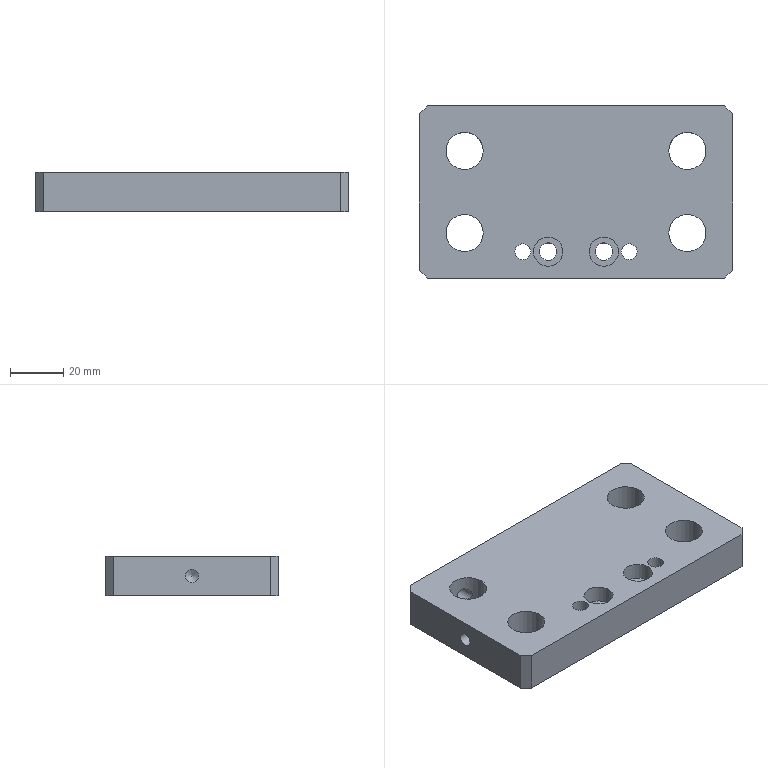Part | NX | features BREP 1 | 1 solid | 26 faces | box 118 x 65 x 15 mm | volume 102149 mm3 | cylinder 13 | plane 12 | cone 1 | commonest cylinder face diameters 14 x4 5 x3 6 x2 6.6 x2 11 x2
STEP:
#1=CARTESIAN_POINT('',(56.,-32.5,0.));
#2=VERTEX_POINT('',#1);
#3=CARTESIAN_POINT('',(59.,-29.5,0.));
#4=VERTEX_POINT('',#3);
#5=CARTESIAN_POINT('',(56.,-32.5,0.));
#6=DIRECTION('',(0.7071,0.7071,0.));
#7=VECTOR('',#6,1000.);
#8=LINE('',#5,#7);
#9=EDGE_CURVE('',#2,#4,#8,.T.);
#10=ORIENTED_EDGE('',*,*,#9,.F.);
#11=CARTESIAN_POINT('',(-56.,-32.5,0.));
#12=VERTEX_POINT('',#11);
#13=CARTESIAN_POINT('',(0.,-32.5,0.));
#14=DIRECTION('',(1.,0.,0.));
#15=VECTOR('',#14,1000.);
#16=LINE('',#13,#15);
#17=EDGE_CURVE('',#12,#2,#16,.T.);
#18=ORIENTED_EDGE('',*,*,#17,.F.);
#19=CARTESIAN_POINT('',(-59.,-29.5,0.));
#20=VERTEX_POINT('',#19);
#21=CARTESIAN_POINT('',(-59.,-29.5,0.));
#22=DIRECTION('',(0.7071,-0.7071,0.));
#23=VECTOR('',#22,1000.);
#24=LINE('',#21,#23);
#25=EDGE_CURVE('',#20,#12,#24,.T.);
#26=ORIENTED_EDGE('',*,*,#25,.F.);
#27=CARTESIAN_POINT('',(-59.,29.5,0.));
#28=VERTEX_POINT('',#27);
#29=CARTESIAN_POINT('',(-59.,0.,0.));
#30=DIRECTION('',(0.,-1.,0.));
#31=VECTOR('',#30,1000.);
#32=LINE('',#29,#31);
#33=EDGE_CURVE('',#28,#20,#32,.T.);
#34=ORIENTED_EDGE('',*,*,#33,.F.);
#35=CARTESIAN_POINT('',(-56.,32.5,0.));
#36=VERTEX_POINT('',#35);
#37=CARTESIAN_POINT('',(-56.,32.5,0.));
#38=DIRECTION('',(-0.7071,-0.7071,0.));
#39=VECTOR('',#38,1000.);
#40=LINE('',#37,#39);
#41=EDGE_CURVE('',#36,#28,#40,.T.);
#42=ORIENTED_EDGE('',*,*,#41,.F.);
#43=CARTESIAN_POINT('',(56.,32.5,0.));
#44=VERTEX_POINT('',#43);
#45=CARTESIAN_POINT('',(0.,32.5,0.));
#46=DIRECTION('',(-1.,0.,0.));
#47=VECTOR('',#46,1000.);
#48=LINE('',#45,#47);
#49=EDGE_CURVE('',#44,#36,#48,.T.);
#50=ORIENTED_EDGE('',*,*,#49,.F.);
#51=CARTESIAN_POINT('',(59.,29.5,0.));
#52=VERTEX_POINT('',#51);
#53=CARTESIAN_POINT('',(59.,29.5,0.));
#54=DIRECTION('',(-0.7071,0.7071,0.));
#55=VECTOR('',#54,1000.);
#56=LINE('',#53,#55);
#57=EDGE_CURVE('',#52,#44,#56,.T.);
#58=ORIENTED_EDGE('',*,*,#57,.F.);
#59=CARTESIAN_POINT('',(59.,0.,0.));
#60=DIRECTION('',(0.,1.,0.));
#61=VECTOR('',#60,1000.);
#62=LINE('',#59,#61);
#63=EDGE_CURVE('',#4,#52,#62,.T.);
#64=ORIENTED_EDGE('',*,*,#63,.F.);
#65=EDGE_LOOP('',(#10,#18,#26,#34,#42,#50,#58,#64));
#66=FACE_BOUND('',#65,.T.);
#67=CARTESIAN_POINT('',(35.,-15.5,0.));
#68=VERTEX_POINT('',#67);
#69=CARTESIAN_POINT('',(42.,-15.5,0.));
#70=DIRECTION('',(0.,0.,-1.));
#71=DIRECTION('',(-1.,0.,0.));
#72=AXIS2_PLACEMENT_3D('',#69,#70,#71);
#73=CIRCLE('',#72,7.);
#74=EDGE_CURVE('',#68,#68,#73,.T.);
#75=ORIENTED_EDGE('',*,*,#74,.F.);
#76=EDGE_LOOP('',(#75));
#77=FACE_BOUND('',#76,.T.);
#78=CARTESIAN_POINT('',(35.,15.5,0.));
#79=VERTEX_POINT('',#78);
#80=CARTESIAN_POINT('',(42.,15.5,0.));
#81=DIRECTION('',(0.,0.,-1.));
#82=DIRECTION('',(-1.,0.,0.));
#83=AXIS2_PLACEMENT_3D('',#80,#81,#82);
#84=CIRCLE('',#83,7.);
#85=EDGE_CURVE('',#79,#79,#84,.T.);
#86=ORIENTED_EDGE('',*,*,#85,.F.);
#87=EDGE_LOOP('',(#86));
#88=FACE_BOUND('',#87,.T.);
#89=CARTESIAN_POINT('',(-49.,15.5,0.));
#90=VERTEX_POINT('',#89);
#91=CARTESIAN_POINT('',(-42.,15.5,0.));
#92=DIRECTION('',(0.,0.,-1.));
#93=DIRECTION('',(-1.,0.,0.));
#94=AXIS2_PLACEMENT_3D('',#91,#92,#93);
#95=CIRCLE('',#94,7.);
#96=EDGE_CURVE('',#90,#90,#95,.T.);
#97=ORIENTED_EDGE('',*,*,#96,.F.);
#98=EDGE_LOOP('',(#97));
#99=FACE_BOUND('',#98,.T.);
#100=CARTESIAN_POINT('',(-49.,-15.5,0.));
#101=VERTEX_POINT('',#100);
#102=CARTESIAN_POINT('',(-42.,-15.5,0.));
#103=DIRECTION('',(0.,0.,-1.));
#104=DIRECTION('',(-1.,0.,0.));
#105=AXIS2_PLACEMENT_3D('',#102,#103,#104);
#106=CIRCLE('',#105,7.);
#107=EDGE_CURVE('',#101,#101,#106,.T.);
#108=ORIENTED_EDGE('',*,*,#107,.F.);
#109=EDGE_LOOP('',(#108));
#110=FACE_BOUND('',#109,.T.);
#111=CARTESIAN_POINT('',(17.,-22.5,0.));
#112=VERTEX_POINT('',#111);
#113=CARTESIAN_POINT('',(20.,-22.5,0.));
#114=DIRECTION('',(0.,0.,-1.));
#115=DIRECTION('',(-1.,0.,0.));
#116=AXIS2_PLACEMENT_3D('',#113,#114,#115);
#117=CIRCLE('',#116,3.);
#118=EDGE_CURVE('',#112,#112,#117,.T.);
#119=ORIENTED_EDGE('',*,*,#118,.F.);
#120=EDGE_LOOP('',(#119));
#121=FACE_BOUND('',#120,.T.);
#122=CARTESIAN_POINT('',(-23.,-22.5,0.));
#123=VERTEX_POINT('',#122);
#124=CARTESIAN_POINT('',(-20.,-22.5,0.));
#125=DIRECTION('',(0.,0.,-1.));
#126=DIRECTION('',(-1.,0.,0.));
#127=AXIS2_PLACEMENT_3D('',#124,#125,#126);
#128=CIRCLE('',#127,3.);
#129=EDGE_CURVE('',#123,#123,#128,.T.);
#130=ORIENTED_EDGE('',*,*,#129,.F.);
#131=EDGE_LOOP('',(#130));
#132=FACE_BOUND('',#131,.T.);
#133=CARTESIAN_POINT('',(13.8,-22.5,0.));
#134=VERTEX_POINT('',#133);
#135=CARTESIAN_POINT('',(10.5,-22.5,0.));
#136=DIRECTION('',(0.,0.,-1.));
#137=DIRECTION('',(1.,0.,0.));
#138=AXIS2_PLACEMENT_3D('',#135,#136,#137);
#139=CIRCLE('',#138,3.3);
#140=EDGE_CURVE('',#134,#134,#139,.T.);
#141=ORIENTED_EDGE('',*,*,#140,.F.);
#142=EDGE_LOOP('',(#141));
#143=FACE_BOUND('',#142,.T.);
#144=CARTESIAN_POINT('',(-7.2,-22.5,0.));
#145=VERTEX_POINT('',#144);
#146=CARTESIAN_POINT('',(-10.5,-22.5,0.));
#147=DIRECTION('',(0.,0.,-1.));
#148=DIRECTION('',(1.,0.,0.));
#149=AXIS2_PLACEMENT_3D('',#146,#147,#148);
#150=CIRCLE('',#149,3.3);
#151=EDGE_CURVE('',#145,#145,#150,.T.);
#152=ORIENTED_EDGE('',*,*,#151,.F.);
#153=EDGE_LOOP('',(#152));
#154=FACE_BOUND('',#153,.T.);
#155=CARTESIAN_POINT('',(0.,0.,0.));
#156=DIRECTION('',(0.,0.,1.));
#157=DIRECTION('',(-1.,0.,0.));
#158=AXIS2_PLACEMENT_3D('',#155,#156,#157);
#159=PLANE('',#158);
#160=ADVANCED_FACE('',(#66,#77,#88,#99,#110,#121,#132,#143,#154),#159,.F.);
#161=CARTESIAN_POINT('',(59.,-29.5,15.));
#162=VERTEX_POINT('',#161);
#163=CARTESIAN_POINT('',(59.,-29.5,15.));
#164=DIRECTION('',(0.,0.,1.));
#165=VECTOR('',#164,1000.);
#166=LINE('',#163,#165);
#167=EDGE_CURVE('',#4,#162,#166,.T.);
#168=ORIENTED_EDGE('',*,*,#167,.F.);
#169=ORIENTED_EDGE('',*,*,#63,.T.);
#170=CARTESIAN_POINT('',(59.,29.5,15.));
#171=VERTEX_POINT('',#170);
#172=CARTESIAN_POINT('',(59.,29.5,15.));
#173=DIRECTION('',(0.,0.,-1.));
#174=VECTOR('',#173,1000.);
#175=LINE('',#172,#174);
#176=EDGE_CURVE('',#171,#52,#175,.T.);
#177=ORIENTED_EDGE('',*,*,#176,.F.);
#178=CARTESIAN_POINT('',(59.,32.5,15.));
#179=DIRECTION('',(0.,1.,0.));
#180=VECTOR('',#179,1000.);
#181=LINE('',#178,#180);
#182=EDGE_CURVE('',#162,#171,#181,.T.);
#183=ORIENTED_EDGE('',*,*,#182,.F.);
#184=EDGE_LOOP('',(#168,#169,#177,#183));
#185=FACE_BOUND('',#184,.T.);
#186=CARTESIAN_POINT('',(59.,32.5,15.));
#187=DIRECTION('',(-1.,0.,0.));
#188=DIRECTION('',(0.,1.,0.));
#189=AXIS2_PLACEMENT_3D('',#186,#187,#188);
#190=PLANE('',#189);
#191=ADVANCED_FACE('',(#185),#190,.F.);
#192=CARTESIAN_POINT('',(56.,-32.5,15.));
#193=VERTEX_POINT('',#192);
#194=CARTESIAN_POINT('',(56.,-32.5,15.));
#195=DIRECTION('',(0.,0.,1.));
#196=VECTOR('',#195,1000.);
#197=LINE('',#194,#196);
#198=EDGE_CURVE('',#2,#193,#197,.T.);
#199=ORIENTED_EDGE('',*,*,#198,.F.);
#200=ORIENTED_EDGE('',*,*,#9,.T.);
#201=ORIENTED_EDGE('',*,*,#167,.T.);
#202=CARTESIAN_POINT('',(59.,-29.5,15.));
#203=DIRECTION('',(0.7071,0.7071,0.));
#204=VECTOR('',#203,1000.);
#205=LINE('',#202,#204);
#206=EDGE_CURVE('',#193,#162,#205,.T.);
#207=ORIENTED_EDGE('',*,*,#206,.F.);
#208=EDGE_LOOP('',(#199,#200,#201,#207));
#209=FACE_BOUND('',#208,.T.);
#210=CARTESIAN_POINT('',(59.,-29.5,15.));
#211=DIRECTION('',(-0.7071,0.7071,0.));
#212=DIRECTION('',(0.7071,0.7071,0.));
#213=AXIS2_PLACEMENT_3D('',#210,#211,#212);
#214=PLANE('',#213);
#215=ADVANCED_FACE('',(#209),#214,.F.);
#216=ORIENTED_EDGE('',*,*,#198,.T.);
#217=CARTESIAN_POINT('',(-56.,-32.5,15.));
#218=VERTEX_POINT('',#217);
#219=CARTESIAN_POINT('',(-59.,-32.5,15.));
#220=DIRECTION('',(1.,0.,0.));
#221=VECTOR('',#220,1000.);
#222=LINE('',#219,#221);
#223=EDGE_CURVE('',#218,#193,#222,.T.);
#224=ORIENTED_EDGE('',*,*,#223,.F.);
#225=CARTESIAN_POINT('',(-56.,-32.5,15.));
#226=DIRECTION('',(0.,0.,1.));
#227=VECTOR('',#226,1000.);
#228=LINE('',#225,#227);
#229=EDGE_CURVE('',#12,#218,#228,.T.);
#230=ORIENTED_EDGE('',*,*,#229,.F.);
#231=ORIENTED_EDGE('',*,*,#17,.T.);
#232=EDGE_LOOP('',(#216,#224,#230,#231));
#233=FACE_BOUND('',#232,.T.);
#234=CARTESIAN_POINT('',(-59.,-32.5,15.));
#235=DIRECTION('',(0.,1.,0.));
#236=DIRECTION('',(0.,0.,-1.));
#237=AXIS2_PLACEMENT_3D('',#234,#235,#236);
#238=PLANE('',#237);
#239=ADVANCED_FACE('',(#233),#238,.F.);
#240=CARTESIAN_POINT('',(-59.,-29.5,15.));
#241=VERTEX_POINT('',#240);
#242=CARTESIAN_POINT('',(-59.,-29.5,15.));
#243=DIRECTION('',(0.,0.,1.));
#244=VECTOR('',#243,1000.);
#245=LINE('',#242,#244);
#246=EDGE_CURVE('',#20,#241,#245,.T.);
#247=ORIENTED_EDGE('',*,*,#246,.F.);
#248=ORIENTED_EDGE('',*,*,#25,.T.);
#249=ORIENTED_EDGE('',*,*,#229,.T.);
#250=CARTESIAN_POINT('',(-56.,-32.5,15.));
#251=DIRECTION('',(0.7071,-0.7071,0.));
#252=VECTOR('',#251,1000.);
#253=LINE('',#250,#252);
#254=EDGE_CURVE('',#241,#218,#253,.T.);
#255=ORIENTED_EDGE('',*,*,#254,.F.);
#256=EDGE_LOOP('',(#247,#248,#249,#255));
#257=FACE_BOUND('',#256,.T.);
#258=CARTESIAN_POINT('',(-56.,-32.5,15.));
#259=DIRECTION('',(0.7071,0.7071,0.));
#260=DIRECTION('',(0.7071,-0.7071,0.));
#261=AXIS2_PLACEMENT_3D('',#258,#259,#260);
#262=PLANE('',#261);
#263=ADVANCED_FACE('',(#257),#262,.F.);
#264=ORIENTED_EDGE('',*,*,#246,.T.);
#265=CARTESIAN_POINT('',(-59.,29.5,15.));
#266=VERTEX_POINT('',#265);
#267=CARTESIAN_POINT('',(-59.,32.5,15.));
#268=DIRECTION('',(0.,-1.,0.));
#269=VECTOR('',#268,1000.);
#270=LINE('',#267,#269);
#271=EDGE_CURVE('',#266,#241,#270,.T.);
#272=ORIENTED_EDGE('',*,*,#271,.F.);
#273=CARTESIAN_POINT('',(-59.,29.5,15.));
#274=DIRECTION('',(0.,0.,1.));
#275=VECTOR('',#274,1000.);
#276=LINE('',#273,#275);
#277=EDGE_CURVE('',#28,#266,#276,.T.);
#278=ORIENTED_EDGE('',*,*,#277,.F.);
#279=ORIENTED_EDGE('',*,*,#33,.T.);
#280=EDGE_LOOP('',(#264,#272,#278,#279));
#281=FACE_BOUND('',#280,.T.);
#282=CARTESIAN_POINT('',(-59.,0.,10.));
#283=VERTEX_POINT('',#282);
#284=CARTESIAN_POINT('',(-59.,0.,7.5));
#285=DIRECTION('',(-1.,0.,0.));
#286=DIRECTION('',(0.,0.,1.));
#287=AXIS2_PLACEMENT_3D('',#284,#285,#286);
#288=CIRCLE('',#287,2.5);
#289=EDGE_CURVE('',#283,#283,#288,.T.);
#290=ORIENTED_EDGE('',*,*,#289,.F.);
#291=EDGE_LOOP('',(#290));
#292=FACE_BOUND('',#291,.T.);
#293=CARTESIAN_POINT('',(-59.,32.5,15.));
#294=DIRECTION('',(1.,0.,0.));
#295=DIRECTION('',(0.,-1.,0.));
#296=AXIS2_PLACEMENT_3D('',#293,#294,#295);
#297=PLANE('',#296);
#298=ADVANCED_FACE('',(#281,#292),#297,.F.);
#299=CARTESIAN_POINT('',(-56.,32.5,15.));
#300=VERTEX_POINT('',#299);
#301=CARTESIAN_POINT('',(-56.,32.5,15.));
#302=DIRECTION('',(0.,0.,1.));
#303=VECTOR('',#302,1000.);
#304=LINE('',#301,#303);
#305=EDGE_CURVE('',#36,#300,#304,.T.);
#306=ORIENTED_EDGE('',*,*,#305,.F.);
#307=ORIENTED_EDGE('',*,*,#41,.T.);
#308=ORIENTED_EDGE('',*,*,#277,.T.);
#309=CARTESIAN_POINT('',(-59.,29.5,15.));
#310=DIRECTION('',(-0.7071,-0.7071,0.));
#311=VECTOR('',#310,1000.);
#312=LINE('',#309,#311);
#313=EDGE_CURVE('',#300,#266,#312,.T.);
#314=ORIENTED_EDGE('',*,*,#313,.F.);
#315=EDGE_LOOP('',(#306,#307,#308,#314));
#316=FACE_BOUND('',#315,.T.);
#317=CARTESIAN_POINT('',(-59.,29.5,15.));
#318=DIRECTION('',(0.7071,-0.7071,0.));
#319=DIRECTION('',(-0.7071,-0.7071,0.));
#320=AXIS2_PLACEMENT_3D('',#317,#318,#319);
#321=PLANE('',#320);
#322=ADVANCED_FACE('',(#316),#321,.F.);
#323=CARTESIAN_POINT('',(56.,32.5,15.));
#324=VERTEX_POINT('',#323);
#325=CARTESIAN_POINT('',(56.,32.5,15.));
#326=DIRECTION('',(0.,0.,1.));
#327=VECTOR('',#326,1000.);
#328=LINE('',#325,#327);
#329=EDGE_CURVE('',#44,#324,#328,.T.);
#330=ORIENTED_EDGE('',*,*,#329,.F.);
#331=ORIENTED_EDGE('',*,*,#49,.T.);
#332=ORIENTED_EDGE('',*,*,#305,.T.);
#333=CARTESIAN_POINT('',(-59.,32.5,15.));
#334=DIRECTION('',(-1.,0.,0.));
#335=VECTOR('',#334,1000.);
#336=LINE('',#333,#335);
#337=EDGE_CURVE('',#324,#300,#336,.T.);
#338=ORIENTED_EDGE('',*,*,#337,.F.);
#339=EDGE_LOOP('',(#330,#331,#332,#338));
#340=FACE_BOUND('',#339,.T.);
#341=CARTESIAN_POINT('',(-38.5,32.5,10.));
#342=VERTEX_POINT('',#341);
#343=CARTESIAN_POINT('',(-38.5,32.5,7.5));
#344=DIRECTION('',(0.,1.,0.));
#345=DIRECTION('',(0.,0.,1.));
#346=AXIS2_PLACEMENT_3D('',#343,#344,#345);
#347=CIRCLE('',#346,2.5);
#348=EDGE_CURVE('',#342,#342,#347,.T.);
#349=ORIENTED_EDGE('',*,*,#348,.F.);
#350=EDGE_LOOP('',(#349));
#351=FACE_BOUND('',#350,.T.);
#352=CARTESIAN_POINT('',(38.5,32.5,10.));
#353=VERTEX_POINT('',#352);
#354=CARTESIAN_POINT('',(38.5,32.5,7.5));
#355=DIRECTION('',(0.,1.,0.));
#356=DIRECTION('',(0.,0.,1.));
#357=AXIS2_PLACEMENT_3D('',#354,#355,#356);
#358=CIRCLE('',#357,2.5);
#359=EDGE_CURVE('',#353,#353,#358,.T.);
#360=ORIENTED_EDGE('',*,*,#359,.F.);
#361=EDGE_LOOP('',(#360));
#362=FACE_BOUND('',#361,.T.);
#363=CARTESIAN_POINT('',(-59.,32.5,15.));
#364=DIRECTION('',(0.,-1.,0.));
#365=DIRECTION('',(0.,0.,1.));
#366=AXIS2_PLACEMENT_3D('',#363,#364,#365);
#367=PLANE('',#366);
#368=ADVANCED_FACE('',(#340,#351,#362),#367,.F.);
#369=ORIENTED_EDGE('',*,*,#176,.T.);
#370=ORIENTED_EDGE('',*,*,#57,.T.);
#371=ORIENTED_EDGE('',*,*,#329,.T.);
#372=CARTESIAN_POINT('',(56.,32.5,15.));
#373=DIRECTION('',(-0.7071,0.7071,0.));
#374=VECTOR('',#373,1000.);
#375=LINE('',#372,#374);
#376=EDGE_CURVE('',#171,#324,#375,.T.);
#377=ORIENTED_EDGE('',*,*,#376,.F.);
#378=EDGE_LOOP('',(#369,#370,#371,#377));
#379=FACE_BOUND('',#378,.T.);
#380=CARTESIAN_POINT('',(56.,32.5,15.));
#381=DIRECTION('',(-0.7071,-0.7071,0.));
#382=DIRECTION('',(-0.7071,0.7071,0.));
#383=AXIS2_PLACEMENT_3D('',#380,#381,#382);
#384=PLANE('',#383);
#385=ADVANCED_FACE('',(#379),#384,.F.);
#386=CARTESIAN_POINT('',(35.,-15.5,15.));
#387=VERTEX_POINT('',#386);
#388=CARTESIAN_POINT('',(42.,-15.5,15.));
#389=DIRECTION('',(0.,0.,-1.));
#390=DIRECTION('',(-1.,0.,0.));
#391=AXIS2_PLACEMENT_3D('',#388,#389,#390);
#392=CIRCLE('',#391,7.);
#393=EDGE_CURVE('',#387,#387,#392,.T.);
#394=ORIENTED_EDGE('',*,*,#393,.F.);
#395=EDGE_LOOP('',(#394));
#396=FACE_BOUND('',#395,.T.);
#397=ORIENTED_EDGE('',*,*,#74,.T.);
#398=EDGE_LOOP('',(#397));
#399=FACE_BOUND('',#398,.T.);
#400=CARTESIAN_POINT('',(42.,-15.5,0.));
#401=DIRECTION('',(0.,0.,-1.));
#402=DIRECTION('',(1.,0.,0.));
#403=AXIS2_PLACEMENT_3D('',#400,#401,#402);
#404=CYLINDRICAL_SURFACE('',#403,7.);
#405=ADVANCED_FACE('',(#396,#399),#404,.F.);
#406=CARTESIAN_POINT('',(35.,15.5,15.));
#407=VERTEX_POINT('',#406);
#408=CARTESIAN_POINT('',(42.,15.5,15.));
#409=DIRECTION('',(0.,0.,-1.));
#410=DIRECTION('',(-1.,0.,0.));
#411=AXIS2_PLACEMENT_3D('',#408,#409,#410);
#412=CIRCLE('',#411,7.);
#413=EDGE_CURVE('',#407,#407,#412,.T.);
#414=ORIENTED_EDGE('',*,*,#413,.F.);
#415=EDGE_LOOP('',(#414));
#416=FACE_BOUND('',#415,.T.);
#417=CARTESIAN_POINT('',(38.5,21.562,5.));
#418=VERTEX_POINT('',#417);
#419=CARTESIAN_POINT('',(37.584,20.964,5.121));
#420=CARTESIAN_POINT('',(38.781,21.8,4.873));
#421=CARTESIAN_POINT('',(40.552,22.412,5.543));
#422=CARTESIAN_POINT('',(41.332,22.458,7.855));
#423=CARTESIAN_POINT('',(40.004,22.31,9.885));
#424=CARTESIAN_POINT('',(38.218,21.475,10.112));
#425=CARTESIAN_POINT('',(37.144,20.573,9.656));
#426=CARTESIAN_POINT('',(36.511,19.877,9.089));
#427=CARTESIAN_POINT('',(36.057,19.211,8.307));
#428=CARTESIAN_POINT('',(35.941,19.007,7.152));
#429=CARTESIAN_POINT('',(36.298,19.588,6.209));
#430=CARTESIAN_POINT('',(36.849,20.272,5.562));
#431=CARTESIAN_POINT('',(37.584,20.964,5.121));
#432=CARTESIAN_POINT('',(38.781,21.8,4.873));
#433=CARTESIAN_POINT('',(40.552,22.412,5.543));
#434=B_SPLINE_CURVE_WITH_KNOTS('',3,(#419,#420,#421,#422,#423,#424,#425,#426,#427,#428,#429,#430,#431,#432,#433),.UNSPECIFIED.,.T.,.F.,(1,1,1,1,1,1,1,1,1,1,1,1,1,1,1,1,1,1,1),(-0.003271,-0.002181,-0.00109,0.,0.002181,0.004362,0.006543,0.008723,0.009814,0.0109,0.01199,0.01309,0.01418,0.01527,0.01636,0.01745,0.01963,0.02181,0.02399),.UNSPECIFIED.);
#435=EDGE_CURVE('',#418,#418,#434,.T.);
#436=ORIENTED_EDGE('',*,*,#435,.F.);
#437=EDGE_LOOP('',(#436));
#438=FACE_BOUND('',#437,.T.);
#439=ORIENTED_EDGE('',*,*,#85,.T.);
#440=EDGE_LOOP('',(#439));
#441=FACE_BOUND('',#440,.T.);
#442=CARTESIAN_POINT('',(42.,15.5,0.));
#443=DIRECTION('',(0.,0.,-1.));
#444=DIRECTION('',(1.,0.,0.));
#445=AXIS2_PLACEMENT_3D('',#442,#443,#444);
#446=CYLINDRICAL_SURFACE('',#445,7.);
#447=ADVANCED_FACE('',(#416,#438,#441),#446,.F.);
#448=CARTESIAN_POINT('',(-49.,15.5,15.));
#449=VERTEX_POINT('',#448);
#450=CARTESIAN_POINT('',(-42.,15.5,15.));
#451=DIRECTION('',(0.,0.,-1.));
#452=DIRECTION('',(-1.,0.,0.));
#453=AXIS2_PLACEMENT_3D('',#450,#451,#452);
#454=CIRCLE('',#453,7.);
#455=EDGE_CURVE('',#449,#449,#454,.T.);
#456=ORIENTED_EDGE('',*,*,#455,.F.);
#457=EDGE_LOOP('',(#456));
#458=FACE_BOUND('',#457,.T.);
#459=CARTESIAN_POINT('',(-38.5,21.562,5.));
#460=VERTEX_POINT('',#459);
#461=CARTESIAN_POINT('',(-40.562,22.415,5.55));
#462=CARTESIAN_POINT('',(-38.777,21.797,4.873));
#463=CARTESIAN_POINT('',(-37.589,20.968,5.119));
#464=CARTESIAN_POINT('',(-36.848,20.271,5.562));
#465=CARTESIAN_POINT('',(-36.297,19.587,6.21));
#466=CARTESIAN_POINT('',(-35.94,19.006,7.157));
#467=CARTESIAN_POINT('',(-36.059,19.213,8.31));
#468=CARTESIAN_POINT('',(-36.514,19.88,9.092));
#469=CARTESIAN_POINT('',(-37.144,20.572,9.655));
#470=CARTESIAN_POINT('',(-38.21,21.469,10.11));
#471=CARTESIAN_POINT('',(-39.988,22.306,9.896));
#472=CARTESIAN_POINT('',(-41.332,22.458,7.866));
#473=CARTESIAN_POINT('',(-40.562,22.415,5.55));
#474=CARTESIAN_POINT('',(-38.777,21.797,4.873));
#475=CARTESIAN_POINT('',(-37.589,20.968,5.119));
#476=B_SPLINE_CURVE_WITH_KNOTS('',3,(#461,#462,#463,#464,#465,#466,#467,#468,#469,#470,#471,#472,#473,#474,#475),.UNSPECIFIED.,.T.,.F.,(1,1,1,1,1,1,1,1,1,1,1,1,1,1,1,1,1,1,1),(-0.006513,-0.004342,-0.002171,0.,0.001085,0.002171,0.003256,0.004342,0.005427,0.006513,0.007598,0.008683,0.01085,0.01303,0.0152,0.01737,0.01845,0.01954,0.02062),.UNSPECIFIED.);
#477=EDGE_CURVE('',#460,#460,#476,.T.);
#478=ORIENTED_EDGE('',*,*,#477,.F.);
#479=EDGE_LOOP('',(#478));
#480=FACE_BOUND('',#479,.T.);
#481=ORIENTED_EDGE('',*,*,#96,.T.);
#482=EDGE_LOOP('',(#481));
#483=FACE_BOUND('',#482,.T.);
#484=CARTESIAN_POINT('',(-42.,15.5,0.));
#485=DIRECTION('',(0.,0.,-1.));
#486=DIRECTION('',(1.,0.,0.));
#487=AXIS2_PLACEMENT_3D('',#484,#485,#486);
#488=CYLINDRICAL_SURFACE('',#487,7.);
#489=ADVANCED_FACE('',(#458,#480,#483),#488,.F.);
#490=CARTESIAN_POINT('',(-49.,-15.5,15.));
#491=VERTEX_POINT('',#490);
#492=CARTESIAN_POINT('',(-42.,-15.5,15.));
#493=DIRECTION('',(0.,0.,-1.));
#494=DIRECTION('',(-1.,0.,0.));
#495=AXIS2_PLACEMENT_3D('',#492,#493,#494);
#496=CIRCLE('',#495,7.);
#497=EDGE_CURVE('',#491,#491,#496,.T.);
#498=ORIENTED_EDGE('',*,*,#497,.F.);
#499=EDGE_LOOP('',(#498));
#500=FACE_BOUND('',#499,.T.);
#501=ORIENTED_EDGE('',*,*,#107,.T.);
#502=EDGE_LOOP('',(#501));
#503=FACE_BOUND('',#502,.T.);
#504=CARTESIAN_POINT('',(-42.,-15.5,0.));
#505=DIRECTION('',(0.,0.,-1.));
#506=DIRECTION('',(1.,0.,0.));
#507=AXIS2_PLACEMENT_3D('',#504,#505,#506);
#508=CYLINDRICAL_SURFACE('',#507,7.);
#509=ADVANCED_FACE('',(#500,#503),#508,.F.);
#510=CARTESIAN_POINT('',(17.,-22.5,15.));
#511=VERTEX_POINT('',#510);
#512=CARTESIAN_POINT('',(20.,-22.5,15.));
#513=DIRECTION('',(0.,0.,-1.));
#514=DIRECTION('',(-1.,0.,0.));
#515=AXIS2_PLACEMENT_3D('',#512,#513,#514);
#516=CIRCLE('',#515,3.);
#517=EDGE_CURVE('',#511,#511,#516,.T.);
#518=ORIENTED_EDGE('',*,*,#517,.F.);
#519=EDGE_LOOP('',(#518));
#520=FACE_BOUND('',#519,.T.);
#521=ORIENTED_EDGE('',*,*,#118,.T.);
#522=EDGE_LOOP('',(#521));
#523=FACE_BOUND('',#522,.T.);
#524=CARTESIAN_POINT('',(20.,-22.5,0.));
#525=DIRECTION('',(0.,0.,-1.));
#526=DIRECTION('',(1.,0.,0.));
#527=AXIS2_PLACEMENT_3D('',#524,#525,#526);
#528=CYLINDRICAL_SURFACE('',#527,3.);
#529=ADVANCED_FACE('',(#520,#523),#528,.F.);
#530=CARTESIAN_POINT('',(-23.,-22.5,15.));
#531=VERTEX_POINT('',#530);
#532=CARTESIAN_POINT('',(-20.,-22.5,15.));
#533=DIRECTION('',(0.,0.,-1.));
#534=DIRECTION('',(-1.,0.,0.));
#535=AXIS2_PLACEMENT_3D('',#532,#533,#534);
#536=CIRCLE('',#535,3.);
#537=EDGE_CURVE('',#531,#531,#536,.T.);
#538=ORIENTED_EDGE('',*,*,#537,.F.);
#539=EDGE_LOOP('',(#538));
#540=FACE_BOUND('',#539,.T.);
#541=ORIENTED_EDGE('',*,*,#129,.T.);
#542=EDGE_LOOP('',(#541));
#543=FACE_BOUND('',#542,.T.);
#544=CARTESIAN_POINT('',(-20.,-22.5,0.));
#545=DIRECTION('',(0.,0.,-1.));
#546=DIRECTION('',(1.,0.,0.));
#547=AXIS2_PLACEMENT_3D('',#544,#545,#546);
#548=CYLINDRICAL_SURFACE('',#547,3.);
#549=ADVANCED_FACE('',(#540,#543),#548,.F.);
#550=ORIENTED_EDGE('',*,*,#140,.T.);
#551=EDGE_LOOP('',(#550));
#552=FACE_BOUND('',#551,.T.);
#553=CARTESIAN_POINT('',(13.8,-22.5,8.6));
#554=VERTEX_POINT('',#553);
#555=CARTESIAN_POINT('',(10.5,-22.5,8.6));
#556=DIRECTION('',(0.,0.,-1.));
#557=DIRECTION('',(1.,0.,0.));
#558=AXIS2_PLACEMENT_3D('',#555,#556,#557);
#559=CIRCLE('',#558,3.3);
#560=EDGE_CURVE('',#554,#554,#559,.T.);
#561=ORIENTED_EDGE('',*,*,#560,.F.);
#562=EDGE_LOOP('',(#561));
#563=FACE_BOUND('',#562,.T.);
#564=CARTESIAN_POINT('',(10.5,-22.5,15.));
#565=DIRECTION('',(0.,0.,1.));
#566=DIRECTION('',(-1.,0.,0.));
#567=AXIS2_PLACEMENT_3D('',#564,#565,#566);
#568=CYLINDRICAL_SURFACE('',#567,3.3);
#569=ADVANCED_FACE('',(#552,#563),#568,.F.);
#570=ORIENTED_EDGE('',*,*,#151,.T.);
#571=EDGE_LOOP('',(#570));
#572=FACE_BOUND('',#571,.T.);
#573=CARTESIAN_POINT('',(-7.2,-22.5,8.6));
#574=VERTEX_POINT('',#573);
#575=CARTESIAN_POINT('',(-10.5,-22.5,8.6));
#576=DIRECTION('',(0.,0.,-1.));
#577=DIRECTION('',(1.,0.,0.));
#578=AXIS2_PLACEMENT_3D('',#575,#576,#577);
#579=CIRCLE('',#578,3.3);
#580=EDGE_CURVE('',#574,#574,#579,.T.);
#581=ORIENTED_EDGE('',*,*,#580,.F.);
#582=EDGE_LOOP('',(#581));
#583=FACE_BOUND('',#582,.T.);
#584=CARTESIAN_POINT('',(-10.5,-22.5,15.));
#585=DIRECTION('',(0.,0.,1.));
#586=DIRECTION('',(-1.,0.,0.));
#587=AXIS2_PLACEMENT_3D('',#584,#585,#586);
#588=CYLINDRICAL_SURFACE('',#587,3.3);
#589=ADVANCED_FACE('',(#572,#583),#588,.F.);
#590=ORIENTED_EDGE('',*,*,#271,.T.);
#591=ORIENTED_EDGE('',*,*,#254,.T.);
#592=ORIENTED_EDGE('',*,*,#223,.T.);
#593=ORIENTED_EDGE('',*,*,#206,.T.);
#594=ORIENTED_EDGE('',*,*,#182,.T.);
#595=ORIENTED_EDGE('',*,*,#376,.T.);
#596=ORIENTED_EDGE('',*,*,#337,.T.);
#597=ORIENTED_EDGE('',*,*,#313,.T.);
#598=EDGE_LOOP('',(#590,#591,#592,#593,#594,#595,#596,#597));
#599=FACE_BOUND('',#598,.T.);
#600=ORIENTED_EDGE('',*,*,#393,.T.);
#601=EDGE_LOOP('',(#600));
#602=FACE_BOUND('',#601,.T.);
#603=ORIENTED_EDGE('',*,*,#413,.T.);
#604=EDGE_LOOP('',(#603));
#605=FACE_BOUND('',#604,.T.);
#606=ORIENTED_EDGE('',*,*,#455,.T.);
#607=EDGE_LOOP('',(#606));
#608=FACE_BOUND('',#607,.T.);
#609=ORIENTED_EDGE('',*,*,#497,.T.);
#610=EDGE_LOOP('',(#609));
#611=FACE_BOUND('',#610,.T.);
#612=ORIENTED_EDGE('',*,*,#517,.T.);
#613=EDGE_LOOP('',(#612));
#614=FACE_BOUND('',#613,.T.);
#615=ORIENTED_EDGE('',*,*,#537,.T.);
#616=EDGE_LOOP('',(#615));
#617=FACE_BOUND('',#616,.T.);
#618=CARTESIAN_POINT('',(16.,-22.5,15.));
#619=VERTEX_POINT('',#618);
#620=CARTESIAN_POINT('',(10.5,-22.5,15.));
#621=DIRECTION('',(0.,0.,-1.));
#622=DIRECTION('',(1.,0.,0.));
#623=AXIS2_PLACEMENT_3D('',#620,#621,#622);
#624=CIRCLE('',#623,5.5);
#625=EDGE_CURVE('',#619,#619,#624,.T.);
#626=ORIENTED_EDGE('',*,*,#625,.T.);
#627=EDGE_LOOP('',(#626));
#628=FACE_BOUND('',#627,.T.);
#629=CARTESIAN_POINT('',(-5.,-22.5,15.));
#630=VERTEX_POINT('',#629);
#631=CARTESIAN_POINT('',(-10.5,-22.5,15.));
#632=DIRECTION('',(0.,0.,-1.));
#633=DIRECTION('',(1.,0.,0.));
#634=AXIS2_PLACEMENT_3D('',#631,#632,#633);
#635=CIRCLE('',#634,5.5);
#636=EDGE_CURVE('',#630,#630,#635,.T.);
#637=ORIENTED_EDGE('',*,*,#636,.T.);
#638=EDGE_LOOP('',(#637));
#639=FACE_BOUND('',#638,.T.);
#640=CARTESIAN_POINT('',(0.,0.,15.));
#641=DIRECTION('',(0.,0.,1.));
#642=DIRECTION('',(-1.,0.,0.));
#643=AXIS2_PLACEMENT_3D('',#640,#641,#642);
#644=PLANE('',#643);
#645=ADVANCED_FACE('',(#599,#602,#605,#608,#611,#614,#617,#628,#639),#644,.T.);
#646=CARTESIAN_POINT('',(-44.,0.,10.));
#647=VERTEX_POINT('',#646);
#648=CARTESIAN_POINT('',(-44.,0.,7.5));
#649=DIRECTION('',(-1.,0.,0.));
#650=DIRECTION('',(0.,0.,1.));
#651=AXIS2_PLACEMENT_3D('',#648,#649,#650);
#652=CIRCLE('',#651,2.5);
#653=EDGE_CURVE('',#647,#647,#652,.T.);
#654=ORIENTED_EDGE('',*,*,#653,.F.);
#655=EDGE_LOOP('',(#654));
#656=FACE_BOUND('',#655,.T.);
#657=ORIENTED_EDGE('',*,*,#289,.T.);
#658=EDGE_LOOP('',(#657));
#659=FACE_BOUND('',#658,.T.);
#660=CARTESIAN_POINT('',(-59.,0.,7.5));
#661=DIRECTION('',(-1.,0.,0.));
#662=DIRECTION('',(0.,0.,-1.));
#663=AXIS2_PLACEMENT_3D('',#660,#661,#662);
#664=CYLINDRICAL_SURFACE('',#663,2.5);
#665=ADVANCED_FACE('',(#656,#659),#664,.F.);
#666=ORIENTED_EDGE('',*,*,#477,.T.);
#667=EDGE_LOOP('',(#666));
#668=FACE_BOUND('',#667,.T.);
#669=ORIENTED_EDGE('',*,*,#348,.T.);
#670=EDGE_LOOP('',(#669));
#671=FACE_BOUND('',#670,.T.);
#672=CARTESIAN_POINT('',(-38.5,32.5,7.5));
#673=DIRECTION('',(0.,1.,0.));
#674=DIRECTION('',(0.,0.,-1.));
#675=AXIS2_PLACEMENT_3D('',#672,#673,#674);
#676=CYLINDRICAL_SURFACE('',#675,2.5);
#677=ADVANCED_FACE('',(#668,#671),#676,.F.);
#678=ORIENTED_EDGE('',*,*,#435,.T.);
#679=EDGE_LOOP('',(#678));
#680=FACE_BOUND('',#679,.T.);
#681=ORIENTED_EDGE('',*,*,#359,.T.);
#682=EDGE_LOOP('',(#681));
#683=FACE_BOUND('',#682,.T.);
#684=CARTESIAN_POINT('',(38.5,32.5,7.5));
#685=DIRECTION('',(0.,1.,0.));
#686=DIRECTION('',(0.,0.,-1.));
#687=AXIS2_PLACEMENT_3D('',#684,#685,#686);
#688=CYLINDRICAL_SURFACE('',#687,2.5);
#689=ADVANCED_FACE('',(#680,#683),#688,.F.);
#690=CARTESIAN_POINT('',(16.,-22.5,8.6));
#691=VERTEX_POINT('',#690);
#692=CARTESIAN_POINT('',(10.5,-22.5,8.6));
#693=DIRECTION('',(0.,0.,-1.));
#694=DIRECTION('',(1.,0.,0.));
#695=AXIS2_PLACEMENT_3D('',#692,#693,#694);
#696=CIRCLE('',#695,5.5);
#697=EDGE_CURVE('',#691,#691,#696,.T.);
#698=ORIENTED_EDGE('',*,*,#697,.F.);
#699=EDGE_LOOP('',(#698));
#700=FACE_BOUND('',#699,.T.);
#701=ORIENTED_EDGE('',*,*,#560,.T.);
#702=EDGE_LOOP('',(#701));
#703=FACE_BOUND('',#702,.T.);
#704=CARTESIAN_POINT('',(13.8,-22.5,8.6));
#705=DIRECTION('',(0.,0.,-1.));
#706=DIRECTION('',(1.,0.,0.));
#707=AXIS2_PLACEMENT_3D('',#704,#705,#706);
#708=PLANE('',#707);
#709=ADVANCED_FACE('',(#700,#703),#708,.F.);
#710=CARTESIAN_POINT('',(-5.,-22.5,8.6));
#711=VERTEX_POINT('',#710);
#712=CARTESIAN_POINT('',(-10.5,-22.5,8.6));
#713=DIRECTION('',(0.,0.,-1.));
#714=DIRECTION('',(1.,0.,0.));
#715=AXIS2_PLACEMENT_3D('',#712,#713,#714);
#716=CIRCLE('',#715,5.5);
#717=EDGE_CURVE('',#711,#711,#716,.T.);
#718=ORIENTED_EDGE('',*,*,#717,.F.);
#719=EDGE_LOOP('',(#718));
#720=FACE_BOUND('',#719,.T.);
#721=ORIENTED_EDGE('',*,*,#580,.T.);
#722=EDGE_LOOP('',(#721));
#723=FACE_BOUND('',#722,.T.);
#724=CARTESIAN_POINT('',(-7.2,-22.5,8.6));
#725=DIRECTION('',(0.,0.,-1.));
#726=DIRECTION('',(1.,0.,0.));
#727=AXIS2_PLACEMENT_3D('',#724,#725,#726);
#728=PLANE('',#727);
#729=ADVANCED_FACE('',(#720,#723),#728,.F.);
#730=ORIENTED_EDGE('',*,*,#625,.F.);
#731=EDGE_LOOP('',(#730));
#732=FACE_BOUND('',#731,.T.);
#733=ORIENTED_EDGE('',*,*,#697,.T.);
#734=EDGE_LOOP('',(#733));
#735=FACE_BOUND('',#734,.T.);
#736=CARTESIAN_POINT('',(10.5,-22.5,15.));
#737=DIRECTION('',(0.,0.,1.));
#738=DIRECTION('',(-1.,0.,0.));
#739=AXIS2_PLACEMENT_3D('',#736,#737,#738);
#740=CYLINDRICAL_SURFACE('',#739,5.5);
#741=ADVANCED_FACE('',(#732,#735),#740,.F.);
#742=ORIENTED_EDGE('',*,*,#636,.F.);
#743=EDGE_LOOP('',(#742));
#744=FACE_BOUND('',#743,.T.);
#745=ORIENTED_EDGE('',*,*,#717,.T.);
#746=EDGE_LOOP('',(#745));
#747=FACE_BOUND('',#746,.T.);
#748=CARTESIAN_POINT('',(-10.5,-22.5,15.));
#749=DIRECTION('',(0.,0.,1.));
#750=DIRECTION('',(-1.,0.,0.));
#751=AXIS2_PLACEMENT_3D('',#748,#749,#750);
#752=CYLINDRICAL_SURFACE('',#751,5.5);
#753=ADVANCED_FACE('',(#744,#747),#752,.F.);
#754=CARTESIAN_POINT('',(-42.498,0.,7.5));
#755=VERTEX_POINT('',#754);
#756=VERTEX_LOOP('',#755);
#757=FACE_BOUND('',#756,.T.);
#758=ORIENTED_EDGE('',*,*,#653,.T.);
#759=EDGE_LOOP('',(#758));
#760=FACE_BOUND('',#759,.T.);
#761=CARTESIAN_POINT('',(-44.,0.,7.5));
#762=DIRECTION('',(-1.,0.,0.));
#763=DIRECTION('',(0.,0.,-1.));
#764=AXIS2_PLACEMENT_3D('',#761,#762,#763);
#765=CONICAL_SURFACE('',#764,2.5,1.03);
#766=ADVANCED_FACE('',(#757,#760),#765,.F.);
#767=CLOSED_SHELL('',(#160,#191,#215,#239,#263,#298,#322,#368,#385,#405,#447,#489,#509,#529,#549,#569,#589,#645,#665,#677,#689,#709,#729,#741,#753,#766));
#768=MANIFOLD_SOLID_BREP('',#767);
#769=(LENGTH_UNIT()NAMED_UNIT(*)SI_UNIT(.MILLI.,.METRE.));
#770=UNCERTAINTY_MEASURE_WITH_UNIT(LENGTH_MEASURE(0.0508),#769,'','');
#771=(NAMED_UNIT(*)PLANE_ANGLE_UNIT()SI_UNIT($,.RADIAN.));
#772=(NAMED_UNIT(*)SI_UNIT($,.STERADIAN.)SOLID_ANGLE_UNIT());
#773=(GEOMETRIC_REPRESENTATION_CONTEXT(3)GLOBAL_UNCERTAINTY_ASSIGNED_CONTEXT((#770))GLOBAL_UNIT_ASSIGNED_CONTEXT((#769,#771,#772))REPRESENTATION_CONTEXT('',''));
#774=ADVANCED_BREP_SHAPE_REPRESENTATION('',(#768),#773);